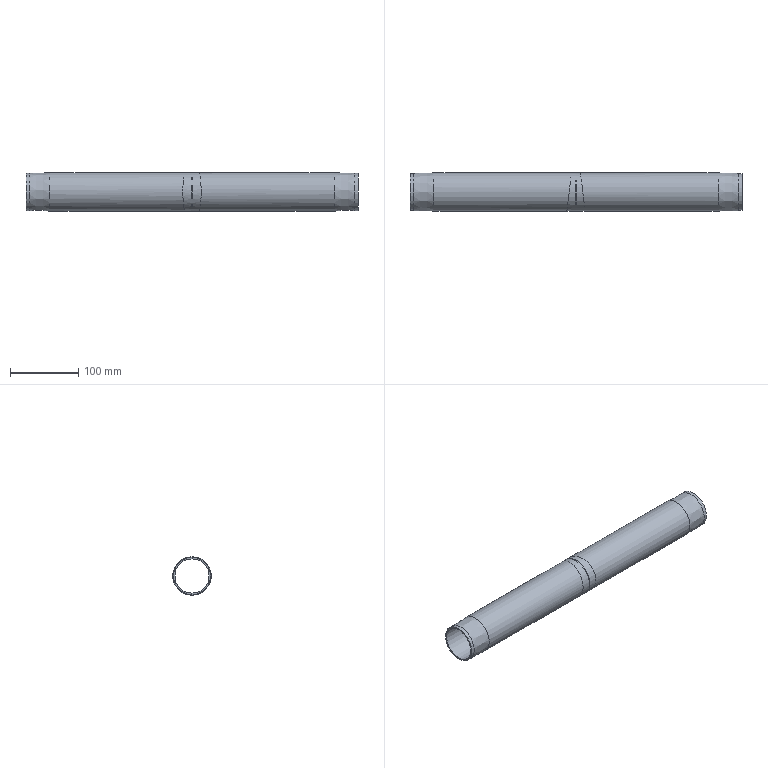Part | STEP file | PN_0050_default | 1 solid | 12 faces | box 485 x 56 x 56 mm | volume 236794 mm3 | cylinder 8 | cone 2 | plane 2 | commonest cylinder face diameters 56 x5 54.429 x2 50 x1
STEP:
#1=CARTESIAN_POINT('',(0.,0.,0.));
#2=DIRECTION('',(0.,0.,1.));
#3=DIRECTION('',(1.,0.,0.));
#4=AXIS2_PLACEMENT_3D('',#1,#2,#3);
#5=CARTESIAN_POINT('',(-0.5,0.,28.));
#6=VERTEX_POINT('',#5);
#7=CARTESIAN_POINT('',(-0.5,0.,0.));
#8=DIRECTION('',(-1.,0.,0.));
#9=DIRECTION('',(0.,0.,1.));
#10=AXIS2_PLACEMENT_3D('',#7,#8,#9);
#11=CIRCLE('',#10,28.);
#12=CARTESIAN_POINT('',(-290.929,0.,0.));
#13=DIRECTION('',(-1.,0.,0.));
#14=DIRECTION('',(0.,0.,1.));
#15=AXIS2_PLACEMENT_3D('',#12,#13,#14);
#16=CYLINDRICAL_SURFACE('',#15,28.);
#17=CARTESIAN_POINT('',(0.,-290.429));
#18=DIRECTION('',(1.,0.));
#19=VECTOR('',#18,1.);
#20=LINE('',#17,#19);
#21=(GEOMETRIC_REPRESENTATION_CONTEXT(2)PARAMETRIC_REPRESENTATION_CONTEXT()REPRESENTATION_CONTEXT('',''));
#22=DEFINITIONAL_REPRESENTATION('',(#20),#21);
#23=PCURVE('',#16,#22);
#24=CARTESIAN_POINT('',(-290.929,0.,0.));
#25=DIRECTION('',(-1.,0.,0.));
#26=DIRECTION('',(0.,0.,1.));
#27=AXIS2_PLACEMENT_3D('',#24,#25,#26);
#28=CYLINDRICAL_SURFACE('',#27,28.);
#29=CARTESIAN_POINT('',(0.,-290.429));
#30=DIRECTION('',(1.,0.));
#31=VECTOR('',#30,1.);
#32=LINE('',#29,#31);
#33=(GEOMETRIC_REPRESENTATION_CONTEXT(2)PARAMETRIC_REPRESENTATION_CONTEXT()REPRESENTATION_CONTEXT('',''));
#34=DEFINITIONAL_REPRESENTATION('',(#32),#33);
#35=PCURVE('',#28,#34);
#36=SURFACE_CURVE('',#11,(#23,#35),.PCURVE_S1.);
#37=EDGE_CURVE('',#6,#6,#36,.T.);
#38=ORIENTED_EDGE('',*,*,#37,.F.);
#39=CARTESIAN_POINT('',(0.5,0.,28.));
#40=VERTEX_POINT('',#39);
#41=CARTESIAN_POINT('',(0.5,0.,28.));
#42=CARTESIAN_POINT('',(-0.5,0.,28.));
#43=B_SPLINE_CURVE_WITH_KNOTS('',1,(#41,#42),.UNSPECIFIED.,.F.,.F.,(2,2),(-291.429,-290.429),.PIECEWISE_BEZIER_KNOTS.);
#44=CARTESIAN_POINT('',(0.,0.));
#45=DIRECTION('',(0.,1.));
#46=VECTOR('',#45,1.);
#47=LINE('',#44,#46);
#48=(GEOMETRIC_REPRESENTATION_CONTEXT(2)PARAMETRIC_REPRESENTATION_CONTEXT()REPRESENTATION_CONTEXT('',''));
#49=DEFINITIONAL_REPRESENTATION('',(#47),#48);
#50=PCURVE('',#16,#49);
#51=CARTESIAN_POINT('',(6.283,0.));
#52=DIRECTION('',(0.,1.));
#53=VECTOR('',#52,1.);
#54=LINE('',#51,#53);
#55=(GEOMETRIC_REPRESENTATION_CONTEXT(2)PARAMETRIC_REPRESENTATION_CONTEXT()REPRESENTATION_CONTEXT('',''));
#56=DEFINITIONAL_REPRESENTATION('',(#54),#55);
#57=PCURVE('',#16,#56);
#58=SEAM_CURVE('',#43,(#50,#57),.PCURVE_S1.);
#59=EDGE_CURVE('',#40,#6,#58,.T.);
#60=ORIENTED_EDGE('',*,*,#59,.F.);
#61=CARTESIAN_POINT('',(0.5,0.,-28.));
#62=VERTEX_POINT('',#61);
#63=CARTESIAN_POINT('',(0.5,0.,0.));
#64=DIRECTION('',(1.,0.,0.));
#65=DIRECTION('',(0.,0.,-1.));
#66=AXIS2_PLACEMENT_3D('',#63,#64,#65);
#67=CIRCLE('',#66,28.);
#68=CARTESIAN_POINT('',(3.142,-291.429));
#69=DIRECTION('',(-1.,0.));
#70=VECTOR('',#69,1.);
#71=LINE('',#68,#70);
#72=(GEOMETRIC_REPRESENTATION_CONTEXT(2)PARAMETRIC_REPRESENTATION_CONTEXT()REPRESENTATION_CONTEXT('',''));
#73=DEFINITIONAL_REPRESENTATION('',(#71),#72);
#74=PCURVE('',#16,#73);
#75=CARTESIAN_POINT('',(-290.929,0.,0.));
#76=DIRECTION('',(-1.,0.,0.));
#77=DIRECTION('',(0.,0.,1.));
#78=AXIS2_PLACEMENT_3D('',#75,#76,#77);
#79=CYLINDRICAL_SURFACE('',#78,28.);
#80=CARTESIAN_POINT('',(3.142,-291.429));
#81=DIRECTION('',(-1.,0.));
#82=VECTOR('',#81,1.);
#83=LINE('',#80,#82);
#84=(GEOMETRIC_REPRESENTATION_CONTEXT(2)PARAMETRIC_REPRESENTATION_CONTEXT()REPRESENTATION_CONTEXT('',''));
#85=DEFINITIONAL_REPRESENTATION('',(#83),#84);
#86=PCURVE('',#79,#85);
#87=SURFACE_CURVE('',#67,(#74,#86),.PCURVE_S1.);
#88=EDGE_CURVE('',#62,#40,#87,.T.);
#89=ORIENTED_EDGE('',*,*,#88,.F.);
#90=CARTESIAN_POINT('',(0.5,0.,0.));
#91=DIRECTION('',(1.,0.,0.));
#92=DIRECTION('',(0.,0.,-1.));
#93=AXIS2_PLACEMENT_3D('',#90,#91,#92);
#94=CIRCLE('',#93,28.);
#95=CARTESIAN_POINT('',(9.425,-291.429));
#96=DIRECTION('',(-1.,0.));
#97=VECTOR('',#96,1.);
#98=LINE('',#95,#97);
#99=(GEOMETRIC_REPRESENTATION_CONTEXT(2)PARAMETRIC_REPRESENTATION_CONTEXT()REPRESENTATION_CONTEXT('',''));
#100=DEFINITIONAL_REPRESENTATION('',(#98),#99);
#101=PCURVE('',#16,#100);
#102=CARTESIAN_POINT('',(9.425,-291.429));
#103=DIRECTION('',(-1.,0.));
#104=VECTOR('',#103,1.);
#105=LINE('',#102,#104);
#106=(GEOMETRIC_REPRESENTATION_CONTEXT(2)PARAMETRIC_REPRESENTATION_CONTEXT()REPRESENTATION_CONTEXT('',''));
#107=DEFINITIONAL_REPRESENTATION('',(#105),#106);
#108=PCURVE('',#79,#107);
#109=SURFACE_CURVE('',#94,(#101,#108),.PCURVE_S1.);
#110=EDGE_CURVE('',#40,#62,#109,.T.);
#111=ORIENTED_EDGE('',*,*,#110,.F.);
#112=ORIENTED_EDGE('',*,*,#59,.T.);
#113=EDGE_LOOP('',(#38,#60,#89,#111,#112));
#114=FACE_BOUND('',#113,.T.);
#115=ADVANCED_FACE('',(#114),#16,.T.);
#116=CARTESIAN_POINT('',(207.5,0.,28.));
#117=VERTEX_POINT('',#116);
#118=CARTESIAN_POINT('',(207.5,0.,0.));
#119=DIRECTION('',(-1.,0.,0.));
#120=DIRECTION('',(0.,0.,1.));
#121=AXIS2_PLACEMENT_3D('',#118,#119,#120);
#122=CIRCLE('',#121,28.);
#123=CARTESIAN_POINT('',(-290.929,0.,0.));
#124=DIRECTION('',(-1.,0.,0.));
#125=DIRECTION('',(0.,0.,1.));
#126=AXIS2_PLACEMENT_3D('',#123,#124,#125);
#127=CYLINDRICAL_SURFACE('',#126,28.);
#128=CARTESIAN_POINT('',(0.,-498.429));
#129=DIRECTION('',(1.,0.));
#130=VECTOR('',#129,1.);
#131=LINE('',#128,#130);
#132=(GEOMETRIC_REPRESENTATION_CONTEXT(2)PARAMETRIC_REPRESENTATION_CONTEXT()REPRESENTATION_CONTEXT('',''));
#133=DEFINITIONAL_REPRESENTATION('',(#131),#132);
#134=PCURVE('',#127,#133);
#135=CARTESIAN_POINT('',(237.5,0.,0.));
#136=DIRECTION('',(-1.,0.,0.));
#137=DIRECTION('',(0.,0.,1.));
#138=AXIS2_PLACEMENT_3D('',#135,#136,#137);
#139=CONICAL_SURFACE('',#138,27.214,0.02618);
#140=CARTESIAN_POINT('',(0.,30.));
#141=DIRECTION('',(1.,0.));
#142=VECTOR('',#141,1.);
#143=LINE('',#140,#142);
#144=(GEOMETRIC_REPRESENTATION_CONTEXT(2)PARAMETRIC_REPRESENTATION_CONTEXT()REPRESENTATION_CONTEXT('',''));
#145=DEFINITIONAL_REPRESENTATION('',(#143),#144);
#146=PCURVE('',#139,#145);
#147=SURFACE_CURVE('',#122,(#134,#146),.PCURVE_S1.);
#148=EDGE_CURVE('',#117,#117,#147,.T.);
#149=ORIENTED_EDGE('',*,*,#148,.T.);
#150=CARTESIAN_POINT('',(9.959,0.,28.));
#151=VERTEX_POINT('',#150);
#152=CARTESIAN_POINT('',(207.5,0.,28.));
#153=CARTESIAN_POINT('',(9.959,0.,28.));
#154=B_SPLINE_CURVE_WITH_KNOTS('',1,(#152,#153),.UNSPECIFIED.,.F.,.F.,(2,2),(-498.429,-300.889),.PIECEWISE_BEZIER_KNOTS.);
#155=CARTESIAN_POINT('',(6.283,0.));
#156=DIRECTION('',(0.,1.));
#157=VECTOR('',#156,1.);
#158=LINE('',#155,#157);
#159=(GEOMETRIC_REPRESENTATION_CONTEXT(2)PARAMETRIC_REPRESENTATION_CONTEXT()REPRESENTATION_CONTEXT('',''));
#160=DEFINITIONAL_REPRESENTATION('',(#158),#159);
#161=PCURVE('',#127,#160);
#162=CARTESIAN_POINT('',(0.,0.));
#163=DIRECTION('',(0.,1.));
#164=VECTOR('',#163,1.);
#165=LINE('',#162,#164);
#166=(GEOMETRIC_REPRESENTATION_CONTEXT(2)PARAMETRIC_REPRESENTATION_CONTEXT()REPRESENTATION_CONTEXT('',''));
#167=DEFINITIONAL_REPRESENTATION('',(#165),#166);
#168=PCURVE('',#127,#167);
#169=SEAM_CURVE('',#154,(#161,#168),.PCURVE_S1.);
#170=EDGE_CURVE('',#117,#151,#169,.T.);
#171=ORIENTED_EDGE('',*,*,#170,.T.);
#172=CARTESIAN_POINT('',(6.587,28.,0.));
#173=VERTEX_POINT('',#172);
#174=CARTESIAN_POINT('',(6.587,28.,0.));
#175=CARTESIAN_POINT('',(6.587,28.,-56.));
#176=CARTESIAN_POINT('',(13.332,-28.,-56.));
#177=CARTESIAN_POINT('',(13.332,-28.,0.));
#178=CARTESIAN_POINT('',(13.332,-28.,56.));
#179=CARTESIAN_POINT('',(6.587,28.,56.));
#180=CARTESIAN_POINT('',(6.587,28.,0.));
#181=(BOUNDED_CURVE()B_SPLINE_CURVE(3,(#174,#175,#176,#177,#178,#179,#180),.UNSPECIFIED.,.T.,.F.)B_SPLINE_CURVE_WITH_KNOTS((1,3,3,3,1),(-3.142,0.,3.142,6.283,9.425),.UNSPECIFIED.)CURVE()GEOMETRIC_REPRESENTATION_ITEM()RATIONAL_B_SPLINE_CURVE((1.,0.3333,0.3333,1.,0.3333,0.3333,1.))REPRESENTATION_ITEM(''));
#182=CARTESIAN_POINT('',(1.571,-297.516));
#183=CARTESIAN_POINT('',(1.631,-297.517));
#184=CARTESIAN_POINT('',(1.764,-297.553));
#185=CARTESIAN_POINT('',(2.001,-297.789));
#186=CARTESIAN_POINT('',(2.281,-298.293));
#187=CARTESIAN_POINT('',(2.604,-299.127));
#188=CARTESIAN_POINT('',(2.958,-300.26));
#189=CARTESIAN_POINT('',(3.325,-301.518));
#190=CARTESIAN_POINT('',(3.679,-302.651));
#191=CARTESIAN_POINT('',(4.002,-303.485));
#192=CARTESIAN_POINT('',(4.282,-303.989));
#193=CARTESIAN_POINT('',(4.521,-304.225));
#194=CARTESIAN_POINT('',(4.712,-304.28));
#195=CARTESIAN_POINT('',(4.904,-304.225));
#196=CARTESIAN_POINT('',(5.143,-303.989));
#197=CARTESIAN_POINT('',(5.423,-303.485));
#198=CARTESIAN_POINT('',(5.745,-302.651));
#199=CARTESIAN_POINT('',(6.1,-301.518));
#200=CARTESIAN_POINT('',(6.467,-300.26));
#201=CARTESIAN_POINT('',(6.821,-299.127));
#202=CARTESIAN_POINT('',(7.143,-298.293));
#203=CARTESIAN_POINT('',(7.424,-297.789));
#204=CARTESIAN_POINT('',(7.661,-297.553));
#205=CARTESIAN_POINT('',(7.794,-297.517));
#206=CARTESIAN_POINT('',(7.854,-297.516));
#207=B_SPLINE_CURVE_WITH_KNOTS('',3,(#182,#183,#184,#185,#186,#187,#188,#189,#190,#191,#192,#193,#194,#195,#196,#197,#198,#199,#200,#201,#202,#203,#204,#205,#206),.UNSPECIFIED.,.F.,.F.,(4,1,1,1,1,1,1,1,1,1,1,1,1,1,1,1,1,1,1,1,1,1,4),(0.,0.2856,0.5712,0.8568,1.142,1.428,1.714,1.999,2.285,2.57,2.856,3.142,3.427,3.713,3.998,4.284,4.57,4.855,5.141,5.426,5.712,5.998,6.283),.QUASI_UNIFORM_KNOTS.);
#208=(GEOMETRIC_REPRESENTATION_CONTEXT(2)PARAMETRIC_REPRESENTATION_CONTEXT()REPRESENTATION_CONTEXT('',''));
#209=DEFINITIONAL_REPRESENTATION('',(#207),#208);
#210=PCURVE('',#127,#209);
#211=CARTESIAN_POINT('',(1.571,-297.516));
#212=CARTESIAN_POINT('',(1.616,-297.517));
#213=CARTESIAN_POINT('',(1.713,-297.537));
#214=CARTESIAN_POINT('',(1.88,-297.659));
#215=CARTESIAN_POINT('',(2.07,-297.908));
#216=CARTESIAN_POINT('',(2.284,-298.317));
#217=CARTESIAN_POINT('',(2.522,-298.91));
#218=CARTESIAN_POINT('',(2.78,-299.681));
#219=CARTESIAN_POINT('',(3.05,-300.577));
#220=CARTESIAN_POINT('',(3.324,-301.508));
#221=CARTESIAN_POINT('',(3.591,-302.371));
#222=CARTESIAN_POINT('',(3.843,-303.086));
#223=CARTESIAN_POINT('',(4.073,-303.617));
#224=CARTESIAN_POINT('',(4.279,-303.969));
#225=CARTESIAN_POINT('',(4.461,-304.171));
#226=CARTESIAN_POINT('',(4.622,-304.259));
#227=CARTESIAN_POINT('',(4.756,-304.269));
#228=CARTESIAN_POINT('',(4.908,-304.212));
#229=CARTESIAN_POINT('',(5.082,-304.051));
#230=CARTESIAN_POINT('',(5.28,-303.753));
#231=CARTESIAN_POINT('',(5.503,-303.283));
#232=CARTESIAN_POINT('',(5.748,-302.629));
#233=CARTESIAN_POINT('',(6.011,-301.807));
#234=CARTESIAN_POINT('',(6.192,-301.198));
#235=CARTESIAN_POINT('',(6.283,-300.889));
#236=B_SPLINE_CURVE_WITH_KNOTS('',3,(#211,#212,#213,#214,#215,#216,#217,#218,#219,#220,#221,#222,#223,#224,#225,#226,#227,#228,#229,#230,#231,#232,#233,#234,#235),.UNSPECIFIED.,.F.,.F.,(4,1,1,1,1,1,1,1,1,1,1,1,1,1,1,1,1,1,1,1,1,1,4),(0.,0.2142,0.4284,0.6426,0.8568,1.071,1.285,1.499,1.714,1.928,2.142,2.356,2.57,2.785,2.999,3.213,3.427,3.641,3.856,4.07,4.284,4.498,4.712),.QUASI_UNIFORM_KNOTS.);
#237=(GEOMETRIC_REPRESENTATION_CONTEXT(2)PARAMETRIC_REPRESENTATION_CONTEXT()REPRESENTATION_CONTEXT('',''));
#238=DEFINITIONAL_REPRESENTATION('',(#236),#237);
#239=PCURVE('',#79,#238);
#240=SURFACE_CURVE('',#181,(#210,#239),.PCURVE_S1.);
#241=EDGE_CURVE('',#173,#151,#240,.T.);
#242=ORIENTED_EDGE('',*,*,#241,.F.);
#243=CARTESIAN_POINT('',(6.587,28.,0.));
#244=CARTESIAN_POINT('',(6.587,28.,-56.));
#245=CARTESIAN_POINT('',(13.332,-28.,-56.));
#246=CARTESIAN_POINT('',(13.332,-28.,0.));
#247=CARTESIAN_POINT('',(13.332,-28.,56.));
#248=CARTESIAN_POINT('',(6.587,28.,56.));
#249=CARTESIAN_POINT('',(6.587,28.,0.));
#250=(BOUNDED_CURVE()B_SPLINE_CURVE(3,(#243,#244,#245,#246,#247,#248,#249),.UNSPECIFIED.,.T.,.F.)B_SPLINE_CURVE_WITH_KNOTS((1,3,3,3,1),(-3.142,0.,3.142,6.283,9.425),.UNSPECIFIED.)CURVE()GEOMETRIC_REPRESENTATION_ITEM()RATIONAL_B_SPLINE_CURVE((1.,0.3333,0.3333,1.,0.3333,0.3333,1.))REPRESENTATION_ITEM(''));
#251=CARTESIAN_POINT('',(-4.712,-297.516));
#252=CARTESIAN_POINT('',(-4.652,-297.517));
#253=CARTESIAN_POINT('',(-4.519,-297.553));
#254=CARTESIAN_POINT('',(-4.282,-297.789));
#255=CARTESIAN_POINT('',(-4.002,-298.293));
#256=CARTESIAN_POINT('',(-3.679,-299.127));
#257=CARTESIAN_POINT('',(-3.325,-300.26));
#258=CARTESIAN_POINT('',(-2.958,-301.518));
#259=CARTESIAN_POINT('',(-2.604,-302.651));
#260=CARTESIAN_POINT('',(-2.281,-303.485));
#261=CARTESIAN_POINT('',(-2.001,-303.989));
#262=CARTESIAN_POINT('',(-1.762,-304.225));
#263=CARTESIAN_POINT('',(-1.571,-304.28));
#264=CARTESIAN_POINT('',(-1.379,-304.225));
#265=CARTESIAN_POINT('',(-1.14,-303.989));
#266=CARTESIAN_POINT('',(-0.8604,-303.485));
#267=CARTESIAN_POINT('',(-0.5378,-302.651));
#268=CARTESIAN_POINT('',(-0.1834,-301.518));
#269=CARTESIAN_POINT('',(0.1834,-300.26));
#270=CARTESIAN_POINT('',(0.5379,-299.127));
#271=CARTESIAN_POINT('',(0.8603,-298.293));
#272=CARTESIAN_POINT('',(1.141,-297.789));
#273=CARTESIAN_POINT('',(1.378,-297.553));
#274=CARTESIAN_POINT('',(1.51,-297.517));
#275=CARTESIAN_POINT('',(1.571,-297.516));
#276=B_SPLINE_CURVE_WITH_KNOTS('',3,(#251,#252,#253,#254,#255,#256,#257,#258,#259,#260,#261,#262,#263,#264,#265,#266,#267,#268,#269,#270,#271,#272,#273,#274,#275),.UNSPECIFIED.,.F.,.F.,(4,1,1,1,1,1,1,1,1,1,1,1,1,1,1,1,1,1,1,1,1,1,4),(0.,0.2856,0.5712,0.8568,1.142,1.428,1.714,1.999,2.285,2.57,2.856,3.142,3.427,3.713,3.998,4.284,4.57,4.855,5.141,5.426,5.712,5.998,6.283),.QUASI_UNIFORM_KNOTS.);
#277=(GEOMETRIC_REPRESENTATION_CONTEXT(2)PARAMETRIC_REPRESENTATION_CONTEXT()REPRESENTATION_CONTEXT('',''));
#278=DEFINITIONAL_REPRESENTATION('',(#276),#277);
#279=PCURVE('',#127,#278);
#280=CARTESIAN_POINT('',(0.000002229,-300.889));
#281=CARTESIAN_POINT('',(0.03031,-300.787));
#282=CARTESIAN_POINT('',(0.09091,-300.582));
#283=CARTESIAN_POINT('',(0.1814,-300.279));
#284=CARTESIAN_POINT('',(0.2712,-299.984));
#285=CARTESIAN_POINT('',(0.3599,-299.699));
#286=CARTESIAN_POINT('',(0.4472,-299.428));
#287=CARTESIAN_POINT('',(0.5328,-299.174));
#288=CARTESIAN_POINT('',(0.6165,-298.937));
#289=CARTESIAN_POINT('',(0.6979,-298.719));
#290=CARTESIAN_POINT('',(0.7771,-298.522));
#291=CARTESIAN_POINT('',(0.8537,-298.344));
#292=CARTESIAN_POINT('',(0.9277,-298.187));
#293=CARTESIAN_POINT('',(0.9991,-298.05));
#294=CARTESIAN_POINT('',(1.068,-297.932));
#295=CARTESIAN_POINT('',(1.134,-297.831));
#296=CARTESIAN_POINT('',(1.197,-297.747));
#297=CARTESIAN_POINT('',(1.258,-297.678));
#298=CARTESIAN_POINT('',(1.316,-297.623));
#299=CARTESIAN_POINT('',(1.372,-297.581));
#300=CARTESIAN_POINT('',(1.425,-297.55));
#301=CARTESIAN_POINT('',(1.476,-297.53));
#302=CARTESIAN_POINT('',(1.525,-297.519));
#303=CARTESIAN_POINT('',(1.556,-297.516));
#304=CARTESIAN_POINT('',(1.571,-297.516));
#305=B_SPLINE_CURVE_WITH_KNOTS('',3,(#280,#281,#282,#283,#284,#285,#286,#287,#288,#289,#290,#291,#292,#293,#294,#295,#296,#297,#298,#299,#300,#301,#302,#303,#304),.UNSPECIFIED.,.F.,.F.,(4,1,1,1,1,1,1,1,1,1,1,1,1,1,1,1,1,1,1,1,1,1,4),(4.712,4.784,4.855,4.927,4.998,5.069,5.141,5.212,5.284,5.355,5.426,5.498,5.569,5.641,5.712,5.783,5.855,5.926,5.998,6.069,6.14,6.212,6.283),.QUASI_UNIFORM_KNOTS.);
#306=(GEOMETRIC_REPRESENTATION_CONTEXT(2)PARAMETRIC_REPRESENTATION_CONTEXT()REPRESENTATION_CONTEXT('',''));
#307=DEFINITIONAL_REPRESENTATION('',(#305),#306);
#308=PCURVE('',#79,#307);
#309=SURFACE_CURVE('',#250,(#279,#308),.PCURVE_S1.);
#310=EDGE_CURVE('',#151,#173,#309,.T.);
#311=ORIENTED_EDGE('',*,*,#310,.F.);
#312=ORIENTED_EDGE('',*,*,#170,.F.);
#313=EDGE_LOOP('',(#149,#171,#242,#311,#312));
#314=FACE_BOUND('',#313,.T.);
#315=ADVANCED_FACE('',(#314),#127,.T.);
#316=CARTESIAN_POINT('',(-207.5,0.,28.));
#317=VERTEX_POINT('',#316);
#318=CARTESIAN_POINT('',(-207.5,0.,0.));
#319=DIRECTION('',(-1.,0.,0.));
#320=DIRECTION('',(0.,0.,1.));
#321=AXIS2_PLACEMENT_3D('',#318,#319,#320);
#322=CIRCLE('',#321,28.);
#323=CARTESIAN_POINT('',(-290.929,0.,0.));
#324=DIRECTION('',(-1.,0.,0.));
#325=DIRECTION('',(0.,0.,1.));
#326=AXIS2_PLACEMENT_3D('',#323,#324,#325);
#327=CYLINDRICAL_SURFACE('',#326,28.);
#328=CARTESIAN_POINT('',(0.,-83.429));
#329=DIRECTION('',(1.,0.));
#330=VECTOR('',#329,1.);
#331=LINE('',#328,#330);
#332=(GEOMETRIC_REPRESENTATION_CONTEXT(2)PARAMETRIC_REPRESENTATION_CONTEXT()REPRESENTATION_CONTEXT('',''));
#333=DEFINITIONAL_REPRESENTATION('',(#331),#332);
#334=PCURVE('',#327,#333);
#335=CARTESIAN_POINT('',(-207.5,0.,0.));
#336=DIRECTION('',(1.,0.,0.));
#337=DIRECTION('',(0.,0.,-1.));
#338=AXIS2_PLACEMENT_3D('',#335,#336,#337);
#339=CONICAL_SURFACE('',#338,28.,0.02618);
#340=CARTESIAN_POINT('',(9.425,0.));
#341=DIRECTION('',(-1.,0.));
#342=VECTOR('',#341,1.);
#343=LINE('',#340,#342);
#344=(GEOMETRIC_REPRESENTATION_CONTEXT(2)PARAMETRIC_REPRESENTATION_CONTEXT()REPRESENTATION_CONTEXT('',''));
#345=DEFINITIONAL_REPRESENTATION('',(#343),#344);
#346=PCURVE('',#339,#345);
#347=SURFACE_CURVE('',#322,(#334,#346),.PCURVE_S1.);
#348=EDGE_CURVE('',#317,#317,#347,.T.);
#349=ORIENTED_EDGE('',*,*,#348,.F.);
#350=CARTESIAN_POINT('',(-9.959,0.,28.));
#351=VERTEX_POINT('',#350);
#352=CARTESIAN_POINT('',(-9.959,0.,28.));
#353=CARTESIAN_POINT('',(-207.5,0.,28.));
#354=B_SPLINE_CURVE_WITH_KNOTS('',1,(#352,#353),.UNSPECIFIED.,.F.,.F.,(2,2),(-280.97,-83.429),.PIECEWISE_BEZIER_KNOTS.);
#355=CARTESIAN_POINT('',(0.,0.));
#356=DIRECTION('',(0.,1.));
#357=VECTOR('',#356,1.);
#358=LINE('',#355,#357);
#359=(GEOMETRIC_REPRESENTATION_CONTEXT(2)PARAMETRIC_REPRESENTATION_CONTEXT()REPRESENTATION_CONTEXT('',''));
#360=DEFINITIONAL_REPRESENTATION('',(#358),#359);
#361=PCURVE('',#327,#360);
#362=CARTESIAN_POINT('',(6.283,0.));
#363=DIRECTION('',(0.,1.));
#364=VECTOR('',#363,1.);
#365=LINE('',#362,#364);
#366=(GEOMETRIC_REPRESENTATION_CONTEXT(2)PARAMETRIC_REPRESENTATION_CONTEXT()REPRESENTATION_CONTEXT('',''));
#367=DEFINITIONAL_REPRESENTATION('',(#365),#366);
#368=PCURVE('',#327,#367);
#369=SEAM_CURVE('',#354,(#361,#368),.PCURVE_S1.);
#370=EDGE_CURVE('',#351,#317,#369,.T.);
#371=ORIENTED_EDGE('',*,*,#370,.F.);
#372=CARTESIAN_POINT('',(-13.332,-28.,0.));
#373=VERTEX_POINT('',#372);
#374=CARTESIAN_POINT('',(-13.332,-28.,0.));
#375=CARTESIAN_POINT('',(-13.332,-28.,-56.));
#376=CARTESIAN_POINT('',(-6.587,28.,-56.));
#377=CARTESIAN_POINT('',(-6.587,28.,0.));
#378=CARTESIAN_POINT('',(-6.587,28.,56.));
#379=CARTESIAN_POINT('',(-13.332,-28.,56.));
#380=CARTESIAN_POINT('',(-13.332,-28.,0.));
#381=(BOUNDED_CURVE()B_SPLINE_CURVE(3,(#374,#375,#376,#377,#378,#379,#380),.UNSPECIFIED.,.T.,.F.)B_SPLINE_CURVE_WITH_KNOTS((1,3,3,3,1),(-3.142,0.,3.142,6.283,9.425),.UNSPECIFIED.)CURVE()GEOMETRIC_REPRESENTATION_ITEM()RATIONAL_B_SPLINE_CURVE((1.,0.3333,0.3333,1.,0.3333,0.3333,1.))REPRESENTATION_ITEM(''));
#382=CARTESIAN_POINT('',(4.712,-277.597));
#383=CARTESIAN_POINT('',(4.652,-277.598));
#384=CARTESIAN_POINT('',(4.519,-277.634));
#385=CARTESIAN_POINT('',(4.282,-277.87));
#386=CARTESIAN_POINT('',(4.002,-278.374));
#387=CARTESIAN_POINT('',(3.679,-279.208));
#388=CARTESIAN_POINT('',(3.325,-280.341));
#389=CARTESIAN_POINT('',(2.958,-281.599));
#390=CARTESIAN_POINT('',(2.604,-282.732));
#391=CARTESIAN_POINT('',(2.281,-283.566));
#392=CARTESIAN_POINT('',(2.001,-284.07));
#393=CARTESIAN_POINT('',(1.762,-284.306));
#394=CARTESIAN_POINT('',(1.571,-284.361));
#395=CARTESIAN_POINT('',(1.379,-284.306));
#396=CARTESIAN_POINT('',(1.14,-284.07));
#397=CARTESIAN_POINT('',(0.8604,-283.566));
#398=CARTESIAN_POINT('',(0.5378,-282.732));
#399=CARTESIAN_POINT('',(0.1834,-281.599));
#400=CARTESIAN_POINT('',(-0.1834,-280.341));
#401=CARTESIAN_POINT('',(-0.5379,-279.208));
#402=CARTESIAN_POINT('',(-0.8603,-278.374));
#403=CARTESIAN_POINT('',(-1.141,-277.87));
#404=CARTESIAN_POINT('',(-1.378,-277.634));
#405=CARTESIAN_POINT('',(-1.51,-277.598));
#406=CARTESIAN_POINT('',(-1.571,-277.597));
#407=B_SPLINE_CURVE_WITH_KNOTS('',3,(#382,#383,#384,#385,#386,#387,#388,#389,#390,#391,#392,#393,#394,#395,#396,#397,#398,#399,#400,#401,#402,#403,#404,#405,#406),.UNSPECIFIED.,.F.,.F.,(4,1,1,1,1,1,1,1,1,1,1,1,1,1,1,1,1,1,1,1,1,1,4),(0.,0.2856,0.5712,0.8568,1.142,1.428,1.714,1.999,2.285,2.57,2.856,3.142,3.427,3.713,3.998,4.284,4.57,4.855,5.141,5.426,5.712,5.998,6.283),.QUASI_UNIFORM_KNOTS.);
#408=(GEOMETRIC_REPRESENTATION_CONTEXT(2)PARAMETRIC_REPRESENTATION_CONTEXT()REPRESENTATION_CONTEXT('',''));
#409=DEFINITIONAL_REPRESENTATION('',(#407),#408);
#410=PCURVE('',#327,#409);
#411=CARTESIAN_POINT('',(4.712,-277.597));
#412=CARTESIAN_POINT('',(4.667,-277.598));
#413=CARTESIAN_POINT('',(4.57,-277.618));
#414=CARTESIAN_POINT('',(4.403,-277.74));
#415=CARTESIAN_POINT('',(4.213,-277.989));
#416=CARTESIAN_POINT('',(3.999,-278.398));
#417=CARTESIAN_POINT('',(3.761,-278.992));
#418=CARTESIAN_POINT('',(3.503,-279.762));
#419=CARTESIAN_POINT('',(3.233,-280.658));
#420=CARTESIAN_POINT('',(2.959,-281.589));
#421=CARTESIAN_POINT('',(2.692,-282.452));
#422=CARTESIAN_POINT('',(2.44,-283.167));
#423=CARTESIAN_POINT('',(2.21,-283.698));
#424=CARTESIAN_POINT('',(2.004,-284.05));
#425=CARTESIAN_POINT('',(1.822,-284.253));
#426=CARTESIAN_POINT('',(1.662,-284.34));
#427=CARTESIAN_POINT('',(1.527,-284.35));
#428=CARTESIAN_POINT('',(1.375,-284.293));
#429=CARTESIAN_POINT('',(1.201,-284.132));
#430=CARTESIAN_POINT('',(1.003,-283.834));
#431=CARTESIAN_POINT('',(0.7804,-283.365));
#432=CARTESIAN_POINT('',(0.5355,-282.71));
#433=CARTESIAN_POINT('',(0.2726,-281.888));
#434=CARTESIAN_POINT('',(0.09109,-281.279));
#435=CARTESIAN_POINT('',(-0.000002229,-280.97));
#436=B_SPLINE_CURVE_WITH_KNOTS('',3,(#411,#412,#413,#414,#415,#416,#417,#418,#419,#420,#421,#422,#423,#424,#425,#426,#427,#428,#429,#430,#431,#432,#433,#434,#435),.UNSPECIFIED.,.F.,.F.,(4,1,1,1,1,1,1,1,1,1,1,1,1,1,1,1,1,1,1,1,1,1,4),(0.,0.2142,0.4284,0.6426,0.8568,1.071,1.285,1.499,1.714,1.928,2.142,2.356,2.57,2.785,2.999,3.213,3.427,3.641,3.856,4.07,4.284,4.498,4.712),.QUASI_UNIFORM_KNOTS.);
#437=(GEOMETRIC_REPRESENTATION_CONTEXT(2)PARAMETRIC_REPRESENTATION_CONTEXT()REPRESENTATION_CONTEXT('',''));
#438=DEFINITIONAL_REPRESENTATION('',(#436),#437);
#439=PCURVE('',#28,#438);
#440=SURFACE_CURVE('',#381,(#410,#439),.PCURVE_S1.);
#441=EDGE_CURVE('',#373,#351,#440,.T.);
#442=ORIENTED_EDGE('',*,*,#441,.F.);
#443=CARTESIAN_POINT('',(-13.332,-28.,0.));
#444=CARTESIAN_POINT('',(-13.332,-28.,-56.));
#445=CARTESIAN_POINT('',(-6.587,28.,-56.));
#446=CARTESIAN_POINT('',(-6.587,28.,0.));
#447=CARTESIAN_POINT('',(-6.587,28.,56.));
#448=CARTESIAN_POINT('',(-13.332,-28.,56.));
#449=CARTESIAN_POINT('',(-13.332,-28.,0.));
#450=(BOUNDED_CURVE()B_SPLINE_CURVE(3,(#443,#444,#445,#446,#447,#448,#449),.UNSPECIFIED.,.T.,.F.)B_SPLINE_CURVE_WITH_KNOTS((1,3,3,3,1),(-3.142,0.,3.142,6.283,9.425),.UNSPECIFIED.)CURVE()GEOMETRIC_REPRESENTATION_ITEM()RATIONAL_B_SPLINE_CURVE((1.,0.3333,0.3333,1.,0.3333,0.3333,1.))REPRESENTATION_ITEM(''));
#451=CARTESIAN_POINT('',(10.996,-277.597));
#452=CARTESIAN_POINT('',(10.935,-277.598));
#453=CARTESIAN_POINT('',(10.803,-277.634));
#454=CARTESIAN_POINT('',(10.565,-277.87));
#455=CARTESIAN_POINT('',(10.285,-278.374));
#456=CARTESIAN_POINT('',(9.963,-279.208));
#457=CARTESIAN_POINT('',(9.608,-280.341));
#458=CARTESIAN_POINT('',(9.241,-281.599));
#459=CARTESIAN_POINT('',(8.887,-282.732));
#460=CARTESIAN_POINT('',(8.564,-283.566));
#461=CARTESIAN_POINT('',(8.285,-284.07));
#462=CARTESIAN_POINT('',(8.045,-284.306));
#463=CARTESIAN_POINT('',(7.854,-284.361));
#464=CARTESIAN_POINT('',(7.663,-284.306));
#465=CARTESIAN_POINT('',(7.423,-284.07));
#466=CARTESIAN_POINT('',(7.144,-283.566));
#467=CARTESIAN_POINT('',(6.821,-282.732));
#468=CARTESIAN_POINT('',(6.467,-281.599));
#469=CARTESIAN_POINT('',(6.1,-280.341));
#470=CARTESIAN_POINT('',(5.745,-279.208));
#471=CARTESIAN_POINT('',(5.423,-278.374));
#472=CARTESIAN_POINT('',(5.143,-277.87));
#473=CARTESIAN_POINT('',(4.905,-277.634));
#474=CARTESIAN_POINT('',(4.773,-277.598));
#475=CARTESIAN_POINT('',(4.712,-277.597));
#476=B_SPLINE_CURVE_WITH_KNOTS('',3,(#451,#452,#453,#454,#455,#456,#457,#458,#459,#460,#461,#462,#463,#464,#465,#466,#467,#468,#469,#470,#471,#472,#473,#474,#475),.UNSPECIFIED.,.F.,.F.,(4,1,1,1,1,1,1,1,1,1,1,1,1,1,1,1,1,1,1,1,1,1,4),(0.,0.2856,0.5712,0.8568,1.142,1.428,1.714,1.999,2.285,2.57,2.856,3.142,3.427,3.713,3.998,4.284,4.57,4.855,5.141,5.426,5.712,5.998,6.283),.QUASI_UNIFORM_KNOTS.);
#477=(GEOMETRIC_REPRESENTATION_CONTEXT(2)PARAMETRIC_REPRESENTATION_CONTEXT()REPRESENTATION_CONTEXT('',''));
#478=DEFINITIONAL_REPRESENTATION('',(#476),#477);
#479=PCURVE('',#327,#478);
#480=CARTESIAN_POINT('',(6.283,-280.97));
#481=CARTESIAN_POINT('',(6.253,-280.868));
#482=CARTESIAN_POINT('',(6.192,-280.663));
#483=CARTESIAN_POINT('',(6.102,-280.36));
#484=CARTESIAN_POINT('',(6.012,-280.065));
#485=CARTESIAN_POINT('',(5.923,-279.78));
#486=CARTESIAN_POINT('',(5.836,-279.51));
#487=CARTESIAN_POINT('',(5.75,-279.255));
#488=CARTESIAN_POINT('',(5.667,-279.018));
#489=CARTESIAN_POINT('',(5.585,-278.8));
#490=CARTESIAN_POINT('',(5.506,-278.603));
#491=CARTESIAN_POINT('',(5.429,-278.426));
#492=CARTESIAN_POINT('',(5.355,-278.269));
#493=CARTESIAN_POINT('',(5.284,-278.131));
#494=CARTESIAN_POINT('',(5.215,-278.013));
#495=CARTESIAN_POINT('',(5.149,-277.912));
#496=CARTESIAN_POINT('',(5.086,-277.828));
#497=CARTESIAN_POINT('',(5.025,-277.759));
#498=CARTESIAN_POINT('',(4.967,-277.704));
#499=CARTESIAN_POINT('',(4.911,-277.662));
#500=CARTESIAN_POINT('',(4.858,-277.632));
#501=CARTESIAN_POINT('',(4.807,-277.611));
#502=CARTESIAN_POINT('',(4.759,-277.6));
#503=CARTESIAN_POINT('',(4.728,-277.597));
#504=CARTESIAN_POINT('',(4.712,-277.597));
#505=B_SPLINE_CURVE_WITH_KNOTS('',3,(#480,#481,#482,#483,#484,#485,#486,#487,#488,#489,#490,#491,#492,#493,#494,#495,#496,#497,#498,#499,#500,#501,#502,#503,#504),.UNSPECIFIED.,.F.,.F.,(4,1,1,1,1,1,1,1,1,1,1,1,1,1,1,1,1,1,1,1,1,1,4),(4.712,4.784,4.855,4.927,4.998,5.069,5.141,5.212,5.284,5.355,5.426,5.498,5.569,5.641,5.712,5.783,5.855,5.926,5.998,6.069,6.14,6.212,6.283),.QUASI_UNIFORM_KNOTS.);
#506=(GEOMETRIC_REPRESENTATION_CONTEXT(2)PARAMETRIC_REPRESENTATION_CONTEXT()REPRESENTATION_CONTEXT('',''));
#507=DEFINITIONAL_REPRESENTATION('',(#505),#506);
#508=PCURVE('',#28,#507);
#509=SURFACE_CURVE('',#450,(#479,#508),.PCURVE_S1.);
#510=EDGE_CURVE('',#351,#373,#509,.T.);
#511=ORIENTED_EDGE('',*,*,#510,.F.);
#512=ORIENTED_EDGE('',*,*,#370,.T.);
#513=EDGE_LOOP('',(#349,#371,#442,#511,#512));
#514=FACE_BOUND('',#513,.T.);
#515=ADVANCED_FACE('',(#514),#327,.T.);
#516=ORIENTED_EDGE('',*,*,#88,.T.);
#517=CARTESIAN_POINT('',(9.959,0.,28.));
#518=CARTESIAN_POINT('',(0.5,0.,28.));
#519=B_SPLINE_CURVE_WITH_KNOTS('',1,(#517,#518),.UNSPECIFIED.,.F.,.F.,(2,2),(-300.889,-291.429),.PIECEWISE_BEZIER_KNOTS.);
#520=CARTESIAN_POINT('',(0.,0.));
#521=DIRECTION('',(0.,1.));
#522=VECTOR('',#521,1.);
#523=LINE('',#520,#522);
#524=(GEOMETRIC_REPRESENTATION_CONTEXT(2)PARAMETRIC_REPRESENTATION_CONTEXT()REPRESENTATION_CONTEXT('',''));
#525=DEFINITIONAL_REPRESENTATION('',(#523),#524);
#526=PCURVE('',#79,#525);
#527=CARTESIAN_POINT('',(6.283,0.));
#528=DIRECTION('',(0.,1.));
#529=VECTOR('',#528,1.);
#530=LINE('',#527,#529);
#531=(GEOMETRIC_REPRESENTATION_CONTEXT(2)PARAMETRIC_REPRESENTATION_CONTEXT()REPRESENTATION_CONTEXT('',''));
#532=DEFINITIONAL_REPRESENTATION('',(#530),#531);
#533=PCURVE('',#79,#532);
#534=SEAM_CURVE('',#519,(#526,#533),.PCURVE_S1.);
#535=EDGE_CURVE('',#151,#40,#534,.T.);
#536=ORIENTED_EDGE('',*,*,#535,.F.);
#537=ORIENTED_EDGE('',*,*,#310,.T.);
#538=ORIENTED_EDGE('',*,*,#241,.T.);
#539=ORIENTED_EDGE('',*,*,#535,.T.);
#540=ORIENTED_EDGE('',*,*,#110,.T.);
#541=EDGE_LOOP('',(#516,#536,#537,#538,#539,#540));
#542=FACE_BOUND('',#541,.T.);
#543=ADVANCED_FACE('',(#542),#79,.T.);
#544=CARTESIAN_POINT('',(-237.5,0.,27.214));
#545=VERTEX_POINT('',#544);
#546=CARTESIAN_POINT('',(-237.5,0.,0.));
#547=DIRECTION('',(-1.,0.,0.));
#548=DIRECTION('',(0.,0.,1.));
#549=AXIS2_PLACEMENT_3D('',#546,#547,#548);
#550=CIRCLE('',#549,27.214);
#551=CARTESIAN_POINT('',(9.425,-30.));
#552=DIRECTION('',(-1.,0.));
#553=VECTOR('',#552,1.);
#554=LINE('',#551,#553);
#555=(GEOMETRIC_REPRESENTATION_CONTEXT(2)PARAMETRIC_REPRESENTATION_CONTEXT()REPRESENTATION_CONTEXT('',''));
#556=DEFINITIONAL_REPRESENTATION('',(#554),#555);
#557=PCURVE('',#339,#556);
#558=CARTESIAN_POINT('',(-290.929,0.,0.));
#559=DIRECTION('',(-1.,0.,0.));
#560=DIRECTION('',(0.,0.,1.));
#561=AXIS2_PLACEMENT_3D('',#558,#559,#560);
#562=CYLINDRICAL_SURFACE('',#561,27.214);
#563=CARTESIAN_POINT('',(0.,-53.429));
#564=DIRECTION('',(1.,0.));
#565=VECTOR('',#564,1.);
#566=LINE('',#563,#565);
#567=(GEOMETRIC_REPRESENTATION_CONTEXT(2)PARAMETRIC_REPRESENTATION_CONTEXT()REPRESENTATION_CONTEXT('',''));
#568=DEFINITIONAL_REPRESENTATION('',(#566),#567);
#569=PCURVE('',#562,#568);
#570=SURFACE_CURVE('',#550,(#557,#569),.PCURVE_S1.);
#571=EDGE_CURVE('',#545,#545,#570,.T.);
#572=ORIENTED_EDGE('',*,*,#571,.F.);
#573=CARTESIAN_POINT('',(-237.5,0.,27.214));
#574=CARTESIAN_POINT('',(-207.5,0.,28.));
#575=B_SPLINE_CURVE_WITH_KNOTS('',1,(#573,#574),.UNSPECIFIED.,.F.,.F.,(2,2),(-30.01,0.),.PIECEWISE_BEZIER_KNOTS.);
#576=CARTESIAN_POINT('',(9.425,0.));
#577=DIRECTION('',(0.,1.));
#578=VECTOR('',#577,1.);
#579=LINE('',#576,#578);
#580=(GEOMETRIC_REPRESENTATION_CONTEXT(2)PARAMETRIC_REPRESENTATION_CONTEXT()REPRESENTATION_CONTEXT('',''));
#581=DEFINITIONAL_REPRESENTATION('',(#579),#580);
#582=PCURVE('',#339,#581);
#583=CARTESIAN_POINT('',(3.142,0.));
#584=DIRECTION('',(0.,1.));
#585=VECTOR('',#584,1.);
#586=LINE('',#583,#585);
#587=(GEOMETRIC_REPRESENTATION_CONTEXT(2)PARAMETRIC_REPRESENTATION_CONTEXT()REPRESENTATION_CONTEXT('',''));
#588=DEFINITIONAL_REPRESENTATION('',(#586),#587);
#589=PCURVE('',#339,#588);
#590=SEAM_CURVE('',#575,(#582,#589),.PCURVE_S1.);
#591=EDGE_CURVE('',#545,#317,#590,.T.);
#592=ORIENTED_EDGE('',*,*,#591,.T.);
#593=ORIENTED_EDGE('',*,*,#348,.T.);
#594=ORIENTED_EDGE('',*,*,#591,.F.);
#595=EDGE_LOOP('',(#572,#592,#593,#594));
#596=FACE_BOUND('',#595,.T.);
#597=ADVANCED_FACE('',(#596),#339,.T.);
#598=CARTESIAN_POINT('',(-242.5,0.,27.214));
#599=VERTEX_POINT('',#598);
#600=CARTESIAN_POINT('',(-242.5,0.,0.));
#601=DIRECTION('',(-1.,0.,0.));
#602=DIRECTION('',(0.,0.,1.));
#603=AXIS2_PLACEMENT_3D('',#600,#601,#602);
#604=CIRCLE('',#603,27.214);
#605=CARTESIAN_POINT('',(0.,-48.429));
#606=DIRECTION('',(1.,0.));
#607=VECTOR('',#606,1.);
#608=LINE('',#605,#607);
#609=(GEOMETRIC_REPRESENTATION_CONTEXT(2)PARAMETRIC_REPRESENTATION_CONTEXT()REPRESENTATION_CONTEXT('',''));
#610=DEFINITIONAL_REPRESENTATION('',(#608),#609);
#611=PCURVE('',#562,#610);
#612=CARTESIAN_POINT('',(-242.5,27.214,0.));
#613=DIRECTION('',(1.,0.,0.));
#614=DIRECTION('',(0.,0.,-1.));
#615=AXIS2_PLACEMENT_3D('',#612,#613,#614);
#616=PLANE('',#615);
#617=CARTESIAN_POINT('',(-27.214,-27.214));
#618=CARTESIAN_POINT('',(-27.214,19.922));
#619=CARTESIAN_POINT('',(13.607,-3.646));
#620=CARTESIAN_POINT('',(54.429,-27.214));
#621=CARTESIAN_POINT('',(13.607,-50.783));
#622=CARTESIAN_POINT('',(-27.214,-74.351));
#623=CARTESIAN_POINT('',(-27.214,-27.214));
#624=(BOUNDED_CURVE()B_SPLINE_CURVE(2,(#617,#618,#619,#620,#621,#622,#623),.UNSPECIFIED.,.T.,.F.)B_SPLINE_CURVE_WITH_KNOTS((1,2,2,2,2,1),(-2.094,0.,2.094,4.189,6.283,8.378),.UNSPECIFIED.)CURVE()GEOMETRIC_REPRESENTATION_ITEM()RATIONAL_B_SPLINE_CURVE((1.,0.5,1.,0.5,1.,0.5,1.))REPRESENTATION_ITEM(''));
#625=(GEOMETRIC_REPRESENTATION_CONTEXT(2)PARAMETRIC_REPRESENTATION_CONTEXT()REPRESENTATION_CONTEXT('',''));
#626=DEFINITIONAL_REPRESENTATION('',(#624),#625);
#627=PCURVE('',#616,#626);
#628=SURFACE_CURVE('',#604,(#611,#627),.PCURVE_S1.);
#629=EDGE_CURVE('',#599,#599,#628,.T.);
#630=ORIENTED_EDGE('',*,*,#629,.F.);
#631=CARTESIAN_POINT('',(-237.5,0.,27.214));
#632=CARTESIAN_POINT('',(-242.5,0.,27.214));
#633=B_SPLINE_CURVE_WITH_KNOTS('',1,(#631,#632),.UNSPECIFIED.,.F.,.F.,(2,2),(-53.429,-48.429),.PIECEWISE_BEZIER_KNOTS.);
#634=CARTESIAN_POINT('',(0.,0.));
#635=DIRECTION('',(0.,1.));
#636=VECTOR('',#635,1.);
#637=LINE('',#634,#636);
#638=(GEOMETRIC_REPRESENTATION_CONTEXT(2)PARAMETRIC_REPRESENTATION_CONTEXT()REPRESENTATION_CONTEXT('',''));
#639=DEFINITIONAL_REPRESENTATION('',(#637),#638);
#640=PCURVE('',#562,#639);
#641=CARTESIAN_POINT('',(6.283,0.));
#642=DIRECTION('',(0.,1.));
#643=VECTOR('',#642,1.);
#644=LINE('',#641,#643);
#645=(GEOMETRIC_REPRESENTATION_CONTEXT(2)PARAMETRIC_REPRESENTATION_CONTEXT()REPRESENTATION_CONTEXT('',''));
#646=DEFINITIONAL_REPRESENTATION('',(#644),#645);
#647=PCURVE('',#562,#646);
#648=SEAM_CURVE('',#633,(#640,#647),.PCURVE_S1.);
#649=EDGE_CURVE('',#545,#599,#648,.T.);
#650=ORIENTED_EDGE('',*,*,#649,.F.);
#651=ORIENTED_EDGE('',*,*,#571,.T.);
#652=ORIENTED_EDGE('',*,*,#649,.T.);
#653=EDGE_LOOP('',(#630,#650,#651,#652));
#654=FACE_BOUND('',#653,.T.);
#655=ADVANCED_FACE('',(#654),#562,.T.);
#656=CARTESIAN_POINT('',(-242.5,0.,25.));
#657=VERTEX_POINT('',#656);
#658=CARTESIAN_POINT('',(-242.5,0.,0.));
#659=DIRECTION('',(-1.,0.,0.));
#660=DIRECTION('',(0.,0.,1.));
#661=AXIS2_PLACEMENT_3D('',#658,#659,#660);
#662=CIRCLE('',#661,25.);
#663=CARTESIAN_POINT('',(-25.,-27.214));
#664=CARTESIAN_POINT('',(-25.,16.087));
#665=CARTESIAN_POINT('',(12.5,-5.564));
#666=CARTESIAN_POINT('',(50.,-27.214));
#667=CARTESIAN_POINT('',(12.5,-48.865));
#668=CARTESIAN_POINT('',(-25.,-70.516));
#669=CARTESIAN_POINT('',(-25.,-27.214));
#670=(BOUNDED_CURVE()B_SPLINE_CURVE(2,(#663,#664,#665,#666,#667,#668,#669),.UNSPECIFIED.,.T.,.F.)B_SPLINE_CURVE_WITH_KNOTS((1,2,2,2,2,1),(-2.094,0.,2.094,4.189,6.283,8.378),.UNSPECIFIED.)CURVE()GEOMETRIC_REPRESENTATION_ITEM()RATIONAL_B_SPLINE_CURVE((1.,0.5,1.,0.5,1.,0.5,1.))REPRESENTATION_ITEM(''));
#671=(GEOMETRIC_REPRESENTATION_CONTEXT(2)PARAMETRIC_REPRESENTATION_CONTEXT()REPRESENTATION_CONTEXT('',''));
#672=DEFINITIONAL_REPRESENTATION('',(#670),#671);
#673=PCURVE('',#616,#672);
#674=CARTESIAN_POINT('',(-290.929,0.,0.));
#675=DIRECTION('',(-1.,0.,0.));
#676=DIRECTION('',(0.,0.,1.));
#677=AXIS2_PLACEMENT_3D('',#674,#675,#676);
#678=CYLINDRICAL_SURFACE('',#677,25.);
#679=CARTESIAN_POINT('',(0.,-48.429));
#680=DIRECTION('',(1.,0.));
#681=VECTOR('',#680,1.);
#682=LINE('',#679,#681);
#683=(GEOMETRIC_REPRESENTATION_CONTEXT(2)PARAMETRIC_REPRESENTATION_CONTEXT()REPRESENTATION_CONTEXT('',''));
#684=DEFINITIONAL_REPRESENTATION('',(#682),#683);
#685=PCURVE('',#678,#684);
#686=SURFACE_CURVE('',#662,(#673,#685),.PCURVE_S1.);
#687=EDGE_CURVE('',#657,#657,#686,.T.);
#688=ORIENTED_EDGE('',*,*,#687,.F.);
#689=EDGE_LOOP('',(#688));
#690=FACE_BOUND('',#689,.T.);
#691=ORIENTED_EDGE('',*,*,#629,.T.);
#692=EDGE_LOOP('',(#691));
#693=FACE_BOUND('',#692,.T.);
#694=ADVANCED_FACE('',(#690,#693),#616,.F.);
#695=CARTESIAN_POINT('',(242.5,0.,25.));
#696=VERTEX_POINT('',#695);
#697=CARTESIAN_POINT('',(242.5,0.,0.));
#698=DIRECTION('',(-1.,0.,0.));
#699=DIRECTION('',(0.,0.,1.));
#700=AXIS2_PLACEMENT_3D('',#697,#698,#699);
#701=CIRCLE('',#700,25.);
#702=CARTESIAN_POINT('',(0.,-533.429));
#703=DIRECTION('',(1.,0.));
#704=VECTOR('',#703,1.);
#705=LINE('',#702,#704);
#706=(GEOMETRIC_REPRESENTATION_CONTEXT(2)PARAMETRIC_REPRESENTATION_CONTEXT()REPRESENTATION_CONTEXT('',''));
#707=DEFINITIONAL_REPRESENTATION('',(#705),#706);
#708=PCURVE('',#678,#707);
#709=CARTESIAN_POINT('',(242.5,27.214,0.));
#710=DIRECTION('',(-1.,0.,0.));
#711=DIRECTION('',(0.,0.,1.));
#712=AXIS2_PLACEMENT_3D('',#709,#710,#711);
#713=PLANE('',#712);
#714=CARTESIAN_POINT('',(0.,-27.214));
#715=DIRECTION('',(1.,0.));
#716=AXIS2_PLACEMENT_2D('',#714,#715);
#717=CIRCLE('',#716,25.);
#718=(GEOMETRIC_REPRESENTATION_CONTEXT(2)PARAMETRIC_REPRESENTATION_CONTEXT()REPRESENTATION_CONTEXT('',''));
#719=DEFINITIONAL_REPRESENTATION('',(#717),#718);
#720=PCURVE('',#713,#719);
#721=SURFACE_CURVE('',#701,(#708,#720),.PCURVE_S1.);
#722=EDGE_CURVE('',#696,#696,#721,.T.);
#723=ORIENTED_EDGE('',*,*,#722,.T.);
#724=CARTESIAN_POINT('',(242.5,0.,25.));
#725=CARTESIAN_POINT('',(-242.5,0.,25.));
#726=B_SPLINE_CURVE_WITH_KNOTS('',1,(#724,#725),.UNSPECIFIED.,.F.,.F.,(2,2),(-533.429,-48.429),.PIECEWISE_BEZIER_KNOTS.);
#727=CARTESIAN_POINT('',(6.283,0.));
#728=DIRECTION('',(0.,1.));
#729=VECTOR('',#728,1.);
#730=LINE('',#727,#729);
#731=(GEOMETRIC_REPRESENTATION_CONTEXT(2)PARAMETRIC_REPRESENTATION_CONTEXT()REPRESENTATION_CONTEXT('',''));
#732=DEFINITIONAL_REPRESENTATION('',(#730),#731);
#733=PCURVE('',#678,#732);
#734=CARTESIAN_POINT('',(0.,0.));
#735=DIRECTION('',(0.,1.));
#736=VECTOR('',#735,1.);
#737=LINE('',#734,#736);
#738=(GEOMETRIC_REPRESENTATION_CONTEXT(2)PARAMETRIC_REPRESENTATION_CONTEXT()REPRESENTATION_CONTEXT('',''));
#739=DEFINITIONAL_REPRESENTATION('',(#737),#738);
#740=PCURVE('',#678,#739);
#741=SEAM_CURVE('',#726,(#733,#740),.PCURVE_S1.);
#742=EDGE_CURVE('',#696,#657,#741,.T.);
#743=ORIENTED_EDGE('',*,*,#742,.T.);
#744=ORIENTED_EDGE('',*,*,#687,.F.);
#745=ORIENTED_EDGE('',*,*,#742,.F.);
#746=EDGE_LOOP('',(#723,#743,#744,#745));
#747=FACE_BOUND('',#746,.F.);
#748=ADVANCED_FACE('',(#747),#678,.F.);
#749=CARTESIAN_POINT('',(242.5,0.,27.214));
#750=VERTEX_POINT('',#749);
#751=CARTESIAN_POINT('',(242.5,0.,0.));
#752=DIRECTION('',(-1.,0.,0.));
#753=DIRECTION('',(0.,0.,1.));
#754=AXIS2_PLACEMENT_3D('',#751,#752,#753);
#755=CIRCLE('',#754,27.214);
#756=CARTESIAN_POINT('',(0.,-27.214));
#757=DIRECTION('',(1.,0.));
#758=AXIS2_PLACEMENT_2D('',#756,#757);
#759=CIRCLE('',#758,27.214);
#760=(GEOMETRIC_REPRESENTATION_CONTEXT(2)PARAMETRIC_REPRESENTATION_CONTEXT()REPRESENTATION_CONTEXT('',''));
#761=DEFINITIONAL_REPRESENTATION('',(#759),#760);
#762=PCURVE('',#713,#761);
#763=CARTESIAN_POINT('',(-290.929,0.,0.));
#764=DIRECTION('',(-1.,0.,0.));
#765=DIRECTION('',(0.,0.,1.));
#766=AXIS2_PLACEMENT_3D('',#763,#764,#765);
#767=CYLINDRICAL_SURFACE('',#766,27.214);
#768=CARTESIAN_POINT('',(0.,-533.429));
#769=DIRECTION('',(1.,0.));
#770=VECTOR('',#769,1.);
#771=LINE('',#768,#770);
#772=(GEOMETRIC_REPRESENTATION_CONTEXT(2)PARAMETRIC_REPRESENTATION_CONTEXT()REPRESENTATION_CONTEXT('',''));
#773=DEFINITIONAL_REPRESENTATION('',(#771),#772);
#774=PCURVE('',#767,#773);
#775=SURFACE_CURVE('',#755,(#762,#774),.PCURVE_S1.);
#776=EDGE_CURVE('',#750,#750,#775,.T.);
#777=ORIENTED_EDGE('',*,*,#776,.F.);
#778=EDGE_LOOP('',(#777));
#779=FACE_BOUND('',#778,.T.);
#780=ORIENTED_EDGE('',*,*,#722,.T.);
#781=EDGE_LOOP('',(#780));
#782=FACE_BOUND('',#781,.T.);
#783=ADVANCED_FACE('',(#779,#782),#713,.F.);
#784=CARTESIAN_POINT('',(237.5,0.,27.214));
#785=VERTEX_POINT('',#784);
#786=CARTESIAN_POINT('',(237.5,0.,0.));
#787=DIRECTION('',(-1.,0.,0.));
#788=DIRECTION('',(0.,0.,1.));
#789=AXIS2_PLACEMENT_3D('',#786,#787,#788);
#790=CIRCLE('',#789,27.214);
#791=CARTESIAN_POINT('',(0.,-528.429));
#792=DIRECTION('',(1.,0.));
#793=VECTOR('',#792,1.);
#794=LINE('',#791,#793);
#795=(GEOMETRIC_REPRESENTATION_CONTEXT(2)PARAMETRIC_REPRESENTATION_CONTEXT()REPRESENTATION_CONTEXT('',''));
#796=DEFINITIONAL_REPRESENTATION('',(#794),#795);
#797=PCURVE('',#767,#796);
#798=CARTESIAN_POINT('',(0.,0.));
#799=DIRECTION('',(1.,0.));
#800=VECTOR('',#799,1.);
#801=LINE('',#798,#800);
#802=(GEOMETRIC_REPRESENTATION_CONTEXT(2)PARAMETRIC_REPRESENTATION_CONTEXT()REPRESENTATION_CONTEXT('',''));
#803=DEFINITIONAL_REPRESENTATION('',(#801),#802);
#804=PCURVE('',#139,#803);
#805=SURFACE_CURVE('',#790,(#797,#804),.PCURVE_S1.);
#806=EDGE_CURVE('',#785,#785,#805,.T.);
#807=ORIENTED_EDGE('',*,*,#806,.F.);
#808=CARTESIAN_POINT('',(242.5,0.,27.214));
#809=CARTESIAN_POINT('',(237.5,0.,27.214));
#810=B_SPLINE_CURVE_WITH_KNOTS('',1,(#808,#809),.UNSPECIFIED.,.F.,.F.,(2,2),(-533.429,-528.429),.PIECEWISE_BEZIER_KNOTS.);
#811=CARTESIAN_POINT('',(0.,0.));
#812=DIRECTION('',(0.,1.));
#813=VECTOR('',#812,1.);
#814=LINE('',#811,#813);
#815=(GEOMETRIC_REPRESENTATION_CONTEXT(2)PARAMETRIC_REPRESENTATION_CONTEXT()REPRESENTATION_CONTEXT('',''));
#816=DEFINITIONAL_REPRESENTATION('',(#814),#815);
#817=PCURVE('',#767,#816);
#818=CARTESIAN_POINT('',(6.283,0.));
#819=DIRECTION('',(0.,1.));
#820=VECTOR('',#819,1.);
#821=LINE('',#818,#820);
#822=(GEOMETRIC_REPRESENTATION_CONTEXT(2)PARAMETRIC_REPRESENTATION_CONTEXT()REPRESENTATION_CONTEXT('',''));
#823=DEFINITIONAL_REPRESENTATION('',(#821),#822);
#824=PCURVE('',#767,#823);
#825=SEAM_CURVE('',#810,(#817,#824),.PCURVE_S1.);
#826=EDGE_CURVE('',#750,#785,#825,.T.);
#827=ORIENTED_EDGE('',*,*,#826,.F.);
#828=ORIENTED_EDGE('',*,*,#776,.T.);
#829=ORIENTED_EDGE('',*,*,#826,.T.);
#830=EDGE_LOOP('',(#807,#827,#828,#829));
#831=FACE_BOUND('',#830,.T.);
#832=ADVANCED_FACE('',(#831),#767,.T.);
#833=ORIENTED_EDGE('',*,*,#148,.F.);
#834=CARTESIAN_POINT('',(237.5,0.,27.214));
#835=CARTESIAN_POINT('',(207.5,0.,28.));
#836=B_SPLINE_CURVE_WITH_KNOTS('',1,(#834,#835),.UNSPECIFIED.,.F.,.F.,(2,2),(0.,30.01),.PIECEWISE_BEZIER_KNOTS.);
#837=CARTESIAN_POINT('',(0.,0.));
#838=DIRECTION('',(0.,1.));
#839=VECTOR('',#838,1.);
#840=LINE('',#837,#839);
#841=(GEOMETRIC_REPRESENTATION_CONTEXT(2)PARAMETRIC_REPRESENTATION_CONTEXT()REPRESENTATION_CONTEXT('',''));
#842=DEFINITIONAL_REPRESENTATION('',(#840),#841);
#843=PCURVE('',#139,#842);
#844=CARTESIAN_POINT('',(6.283,0.));
#845=DIRECTION('',(0.,1.));
#846=VECTOR('',#845,1.);
#847=LINE('',#844,#846);
#848=(GEOMETRIC_REPRESENTATION_CONTEXT(2)PARAMETRIC_REPRESENTATION_CONTEXT()REPRESENTATION_CONTEXT('',''));
#849=DEFINITIONAL_REPRESENTATION('',(#847),#848);
#850=PCURVE('',#139,#849);
#851=SEAM_CURVE('',#836,(#843,#850),.PCURVE_S1.);
#852=EDGE_CURVE('',#785,#117,#851,.T.);
#853=ORIENTED_EDGE('',*,*,#852,.F.);
#854=ORIENTED_EDGE('',*,*,#806,.T.);
#855=ORIENTED_EDGE('',*,*,#852,.T.);
#856=EDGE_LOOP('',(#833,#853,#854,#855));
#857=FACE_BOUND('',#856,.T.);
#858=ADVANCED_FACE('',(#857),#139,.T.);
#859=ORIENTED_EDGE('',*,*,#441,.T.);
#860=CARTESIAN_POINT('',(-0.5,0.,28.));
#861=CARTESIAN_POINT('',(-9.959,0.,28.));
#862=B_SPLINE_CURVE_WITH_KNOTS('',1,(#860,#861),.UNSPECIFIED.,.F.,.F.,(2,2),(-290.429,-280.97),.PIECEWISE_BEZIER_KNOTS.);
#863=CARTESIAN_POINT('',(0.,0.));
#864=DIRECTION('',(0.,1.));
#865=VECTOR('',#864,1.);
#866=LINE('',#863,#865);
#867=(GEOMETRIC_REPRESENTATION_CONTEXT(2)PARAMETRIC_REPRESENTATION_CONTEXT()REPRESENTATION_CONTEXT('',''));
#868=DEFINITIONAL_REPRESENTATION('',(#866),#867);
#869=PCURVE('',#28,#868);
#870=CARTESIAN_POINT('',(6.283,0.));
#871=DIRECTION('',(0.,1.));
#872=VECTOR('',#871,1.);
#873=LINE('',#870,#872);
#874=(GEOMETRIC_REPRESENTATION_CONTEXT(2)PARAMETRIC_REPRESENTATION_CONTEXT()REPRESENTATION_CONTEXT('',''));
#875=DEFINITIONAL_REPRESENTATION('',(#873),#874);
#876=PCURVE('',#28,#875);
#877=SEAM_CURVE('',#862,(#869,#876),.PCURVE_S1.);
#878=EDGE_CURVE('',#6,#351,#877,.T.);
#879=ORIENTED_EDGE('',*,*,#878,.F.);
#880=ORIENTED_EDGE('',*,*,#37,.T.);
#881=ORIENTED_EDGE('',*,*,#878,.T.);
#882=ORIENTED_EDGE('',*,*,#510,.T.);
#883=EDGE_LOOP('',(#859,#879,#880,#881,#882));
#884=FACE_BOUND('',#883,.T.);
#885=ADVANCED_FACE('',(#884),#28,.T.);
#886=CLOSED_SHELL('',(#115,#315,#515,#543,#597,#655,#694,#748,#783,#832,#858,#885));
#887=MANIFOLD_SOLID_BREP('',#886);
#888=(LENGTH_UNIT()NAMED_UNIT(*)SI_UNIT(.MILLI.,.METRE.));
#889=UNCERTAINTY_MEASURE_WITH_UNIT(LENGTH_MEASURE(0.01),#888,'','');
#890=(NAMED_UNIT(*)PLANE_ANGLE_UNIT()SI_UNIT($,.RADIAN.));
#891=(NAMED_UNIT(*)SI_UNIT($,.STERADIAN.)SOLID_ANGLE_UNIT());
#892=(GEOMETRIC_REPRESENTATION_CONTEXT(3)GLOBAL_UNCERTAINTY_ASSIGNED_CONTEXT((#889))GLOBAL_UNIT_ASSIGNED_CONTEXT((#888,#890,#891))REPRESENTATION_CONTEXT('',''));
#893=ADVANCED_BREP_SHAPE_REPRESENTATION('',(#4,#887),#892);